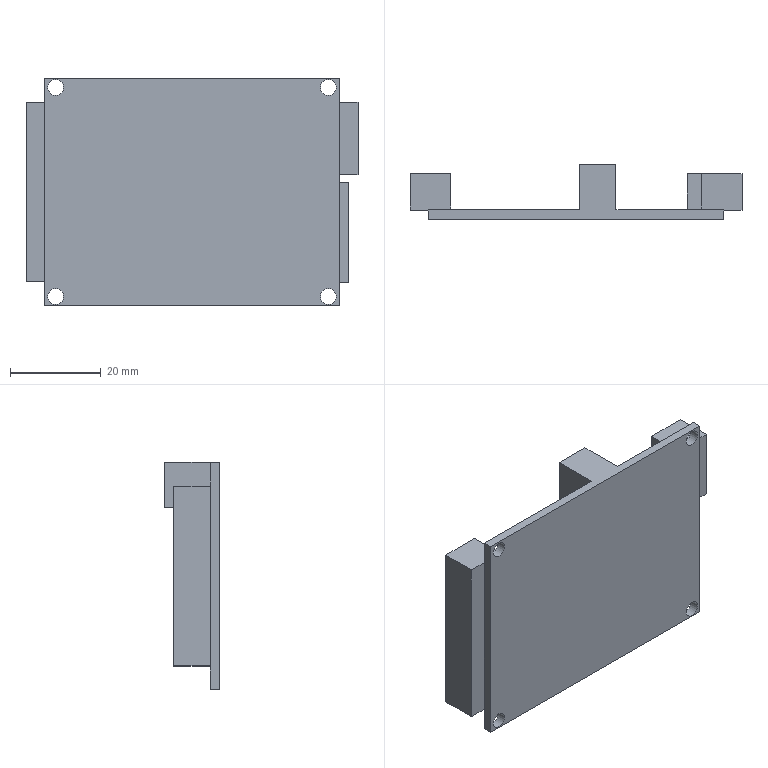Part | NX | features BREP 1 | 1 solid | 32 faces | box 73 x 12 x 50 mm | volume 12980 mm3 | plane 28 | cylinder 4 | commonest cylinder face diameters 3.5 x4
STEP:
#1=CARTESIAN_POINT('',(30.,2.,21.25));
#2=VERTEX_POINT('',#1);
#3=CARTESIAN_POINT('',(30.,2.,23.));
#4=DIRECTION('',(0.,1.,0.));
#5=DIRECTION('',(0.,0.,-1.));
#6=AXIS2_PLACEMENT_3D('',#3,#4,#5);
#7=CIRCLE('',#6,1.75);
#8=EDGE_CURVE('',#2,#2,#7,.T.);
#9=ORIENTED_EDGE('',*,*,#8,.T.);
#10=EDGE_LOOP('',(#9));
#11=FACE_BOUND('',#10,.T.);
#12=CARTESIAN_POINT('',(30.,0.,21.25));
#13=VERTEX_POINT('',#12);
#14=CARTESIAN_POINT('',(30.,0.,23.));
#15=DIRECTION('',(0.,1.,0.));
#16=DIRECTION('',(0.,0.,-1.));
#17=AXIS2_PLACEMENT_3D('',#14,#15,#16);
#18=CIRCLE('',#17,1.75);
#19=EDGE_CURVE('',#13,#13,#18,.T.);
#20=ORIENTED_EDGE('',*,*,#19,.F.);
#21=EDGE_LOOP('',(#20));
#22=FACE_BOUND('',#21,.T.);
#23=CARTESIAN_POINT('',(30.,0.,23.));
#24=DIRECTION('',(0.,1.,0.));
#25=DIRECTION('',(0.,0.,1.));
#26=AXIS2_PLACEMENT_3D('',#23,#24,#25);
#27=CYLINDRICAL_SURFACE('',#26,1.75);
#28=ADVANCED_FACE('',(#11,#22),#27,.F.);
#29=CARTESIAN_POINT('',(-30.,2.,24.75));
#30=VERTEX_POINT('',#29);
#31=CARTESIAN_POINT('',(-30.,2.,23.));
#32=DIRECTION('',(0.,1.,0.));
#33=DIRECTION('',(0.,0.,1.));
#34=AXIS2_PLACEMENT_3D('',#31,#32,#33);
#35=CIRCLE('',#34,1.75);
#36=EDGE_CURVE('',#30,#30,#35,.T.);
#37=ORIENTED_EDGE('',*,*,#36,.T.);
#38=EDGE_LOOP('',(#37));
#39=FACE_BOUND('',#38,.T.);
#40=CARTESIAN_POINT('',(-30.,0.,24.75));
#41=VERTEX_POINT('',#40);
#42=CARTESIAN_POINT('',(-30.,0.,23.));
#43=DIRECTION('',(0.,1.,0.));
#44=DIRECTION('',(0.,0.,1.));
#45=AXIS2_PLACEMENT_3D('',#42,#43,#44);
#46=CIRCLE('',#45,1.75);
#47=EDGE_CURVE('',#41,#41,#46,.T.);
#48=ORIENTED_EDGE('',*,*,#47,.F.);
#49=EDGE_LOOP('',(#48));
#50=FACE_BOUND('',#49,.T.);
#51=CARTESIAN_POINT('',(-30.,0.,23.));
#52=DIRECTION('',(0.,1.,0.));
#53=DIRECTION('',(0.,0.,1.));
#54=AXIS2_PLACEMENT_3D('',#51,#52,#53);
#55=CYLINDRICAL_SURFACE('',#54,1.75);
#56=ADVANCED_FACE('',(#39,#50),#55,.F.);
#57=CARTESIAN_POINT('',(-30.,2.,-24.75));
#58=VERTEX_POINT('',#57);
#59=CARTESIAN_POINT('',(-30.,2.,-23.));
#60=DIRECTION('',(0.,1.,0.));
#61=DIRECTION('',(0.,0.,-1.));
#62=AXIS2_PLACEMENT_3D('',#59,#60,#61);
#63=CIRCLE('',#62,1.75);
#64=EDGE_CURVE('',#58,#58,#63,.T.);
#65=ORIENTED_EDGE('',*,*,#64,.T.);
#66=EDGE_LOOP('',(#65));
#67=FACE_BOUND('',#66,.T.);
#68=CARTESIAN_POINT('',(-30.,0.,-24.75));
#69=VERTEX_POINT('',#68);
#70=CARTESIAN_POINT('',(-30.,0.,-23.));
#71=DIRECTION('',(0.,1.,0.));
#72=DIRECTION('',(0.,0.,-1.));
#73=AXIS2_PLACEMENT_3D('',#70,#71,#72);
#74=CIRCLE('',#73,1.75);
#75=EDGE_CURVE('',#69,#69,#74,.T.);
#76=ORIENTED_EDGE('',*,*,#75,.F.);
#77=EDGE_LOOP('',(#76));
#78=FACE_BOUND('',#77,.T.);
#79=CARTESIAN_POINT('',(-30.,0.,-23.));
#80=DIRECTION('',(0.,1.,0.));
#81=DIRECTION('',(0.,0.,1.));
#82=AXIS2_PLACEMENT_3D('',#79,#80,#81);
#83=CYLINDRICAL_SURFACE('',#82,1.75);
#84=ADVANCED_FACE('',(#67,#78),#83,.F.);
#85=CARTESIAN_POINT('',(30.,2.,-21.25));
#86=VERTEX_POINT('',#85);
#87=CARTESIAN_POINT('',(30.,2.,-23.));
#88=DIRECTION('',(0.,1.,0.));
#89=DIRECTION('',(0.,0.,1.));
#90=AXIS2_PLACEMENT_3D('',#87,#88,#89);
#91=CIRCLE('',#90,1.75);
#92=EDGE_CURVE('',#86,#86,#91,.T.);
#93=ORIENTED_EDGE('',*,*,#92,.T.);
#94=EDGE_LOOP('',(#93));
#95=FACE_BOUND('',#94,.T.);
#96=CARTESIAN_POINT('',(30.,0.,-21.25));
#97=VERTEX_POINT('',#96);
#98=CARTESIAN_POINT('',(30.,0.,-23.));
#99=DIRECTION('',(0.,1.,0.));
#100=DIRECTION('',(0.,0.,1.));
#101=AXIS2_PLACEMENT_3D('',#98,#99,#100);
#102=CIRCLE('',#101,1.75);
#103=EDGE_CURVE('',#97,#97,#102,.T.);
#104=ORIENTED_EDGE('',*,*,#103,.F.);
#105=EDGE_LOOP('',(#104));
#106=FACE_BOUND('',#105,.T.);
#107=CARTESIAN_POINT('',(30.,0.,-23.));
#108=DIRECTION('',(0.,1.,0.));
#109=DIRECTION('',(0.,0.,1.));
#110=AXIS2_PLACEMENT_3D('',#107,#108,#109);
#111=CYLINDRICAL_SURFACE('',#110,1.75);
#112=ADVANCED_FACE('',(#95,#106),#111,.F.);
#113=ORIENTED_EDGE('',*,*,#92,.F.);
#114=EDGE_LOOP('',(#113));
#115=FACE_BOUND('',#114,.T.);
#116=ORIENTED_EDGE('',*,*,#64,.F.);
#117=EDGE_LOOP('',(#116));
#118=FACE_BOUND('',#117,.T.);
#119=ORIENTED_EDGE('',*,*,#36,.F.);
#120=EDGE_LOOP('',(#119));
#121=FACE_BOUND('',#120,.T.);
#122=ORIENTED_EDGE('',*,*,#8,.F.);
#123=EDGE_LOOP('',(#122));
#124=FACE_BOUND('',#123,.T.);
#125=CARTESIAN_POINT('',(-32.5,2.,25.));
#126=VERTEX_POINT('',#125);
#127=CARTESIAN_POINT('',(0.7928,2.,25.));
#128=VERTEX_POINT('',#127);
#129=CARTESIAN_POINT('',(-32.5,2.,25.));
#130=DIRECTION('',(1.,0.,0.));
#131=VECTOR('',#130,1000.);
#132=LINE('',#129,#131);
#133=EDGE_CURVE('',#126,#128,#132,.T.);
#134=ORIENTED_EDGE('',*,*,#133,.T.);
#135=CARTESIAN_POINT('',(0.7928,2.,15.));
#136=VERTEX_POINT('',#135);
#137=CARTESIAN_POINT('',(0.7928,2.,15.));
#138=DIRECTION('',(0.,0.,1.));
#139=VECTOR('',#138,1000.);
#140=LINE('',#137,#139);
#141=EDGE_CURVE('',#136,#128,#140,.T.);
#142=ORIENTED_EDGE('',*,*,#141,.F.);
#143=CARTESIAN_POINT('',(8.793,2.,15.));
#144=VERTEX_POINT('',#143);
#145=CARTESIAN_POINT('',(0.7928,2.,15.));
#146=DIRECTION('',(-1.,0.,0.));
#147=VECTOR('',#146,1000.);
#148=LINE('',#145,#147);
#149=EDGE_CURVE('',#144,#136,#148,.T.);
#150=ORIENTED_EDGE('',*,*,#149,.F.);
#151=CARTESIAN_POINT('',(8.793,2.,25.));
#152=VERTEX_POINT('',#151);
#153=CARTESIAN_POINT('',(8.793,2.,15.));
#154=DIRECTION('',(0.,0.,-1.));
#155=VECTOR('',#154,1000.);
#156=LINE('',#153,#155);
#157=EDGE_CURVE('',#152,#144,#156,.T.);
#158=ORIENTED_EDGE('',*,*,#157,.F.);
#159=CARTESIAN_POINT('',(32.5,2.,25.));
#160=VERTEX_POINT('',#159);
#161=CARTESIAN_POINT('',(-32.5,2.,25.));
#162=DIRECTION('',(1.,0.,0.));
#163=VECTOR('',#162,1000.);
#164=LINE('',#161,#163);
#165=EDGE_CURVE('',#152,#160,#164,.T.);
#166=ORIENTED_EDGE('',*,*,#165,.T.);
#167=CARTESIAN_POINT('',(32.5,2.,19.756));
#168=VERTEX_POINT('',#167);
#169=CARTESIAN_POINT('',(32.5,2.,-25.));
#170=DIRECTION('',(0.,0.,-1.));
#171=VECTOR('',#170,1000.);
#172=LINE('',#169,#171);
#173=EDGE_CURVE('',#160,#168,#172,.T.);
#174=ORIENTED_EDGE('',*,*,#173,.T.);
#175=CARTESIAN_POINT('',(27.5,2.,19.756));
#176=VERTEX_POINT('',#175);
#177=CARTESIAN_POINT('',(27.5,2.,19.756));
#178=DIRECTION('',(1.,0.,0.));
#179=VECTOR('',#178,1000.);
#180=LINE('',#177,#179);
#181=EDGE_CURVE('',#176,#168,#180,.T.);
#182=ORIENTED_EDGE('',*,*,#181,.F.);
#183=CARTESIAN_POINT('',(27.5,2.,3.756));
#184=VERTEX_POINT('',#183);
#185=CARTESIAN_POINT('',(27.5,2.,19.756));
#186=DIRECTION('',(0.,0.,1.));
#187=VECTOR('',#186,1000.);
#188=LINE('',#185,#187);
#189=EDGE_CURVE('',#184,#176,#188,.T.);
#190=ORIENTED_EDGE('',*,*,#189,.F.);
#191=CARTESIAN_POINT('',(32.5,2.,3.756));
#192=VERTEX_POINT('',#191);
#193=CARTESIAN_POINT('',(0.,2.,3.756));
#194=DIRECTION('',(1.,0.,0.));
#195=VECTOR('',#194,1000.);
#196=LINE('',#193,#195);
#197=EDGE_CURVE('',#184,#192,#196,.T.);
#198=ORIENTED_EDGE('',*,*,#197,.T.);
#199=CARTESIAN_POINT('',(32.5,2.,2.163));
#200=VERTEX_POINT('',#199);
#201=CARTESIAN_POINT('',(32.5,2.,-25.));
#202=DIRECTION('',(0.,0.,-1.));
#203=VECTOR('',#202,1000.);
#204=LINE('',#201,#203);
#205=EDGE_CURVE('',#192,#200,#204,.T.);
#206=ORIENTED_EDGE('',*,*,#205,.T.);
#207=CARTESIAN_POINT('',(24.5,2.,2.163));
#208=VERTEX_POINT('',#207);
#209=CARTESIAN_POINT('',(24.5,2.,2.163));
#210=DIRECTION('',(1.,0.,0.));
#211=VECTOR('',#210,1000.);
#212=LINE('',#209,#211);
#213=EDGE_CURVE('',#208,#200,#212,.T.);
#214=ORIENTED_EDGE('',*,*,#213,.F.);
#215=CARTESIAN_POINT('',(24.5,2.,-19.837));
#216=VERTEX_POINT('',#215);
#217=CARTESIAN_POINT('',(24.5,2.,-19.837));
#218=DIRECTION('',(0.,0.,1.));
#219=VECTOR('',#218,1000.);
#220=LINE('',#217,#219);
#221=EDGE_CURVE('',#216,#208,#220,.T.);
#222=ORIENTED_EDGE('',*,*,#221,.F.);
#223=CARTESIAN_POINT('',(32.5,2.,-19.837));
#224=VERTEX_POINT('',#223);
#225=CARTESIAN_POINT('',(24.5,2.,-19.837));
#226=DIRECTION('',(-1.,0.,0.));
#227=VECTOR('',#226,1000.);
#228=LINE('',#225,#227);
#229=EDGE_CURVE('',#224,#216,#228,.T.);
#230=ORIENTED_EDGE('',*,*,#229,.F.);
#231=CARTESIAN_POINT('',(32.5,2.,-25.));
#232=VERTEX_POINT('',#231);
#233=CARTESIAN_POINT('',(32.5,2.,-25.));
#234=DIRECTION('',(0.,0.,-1.));
#235=VECTOR('',#234,1000.);
#236=LINE('',#233,#235);
#237=EDGE_CURVE('',#224,#232,#236,.T.);
#238=ORIENTED_EDGE('',*,*,#237,.T.);
#239=CARTESIAN_POINT('',(-32.5,2.,-25.));
#240=VERTEX_POINT('',#239);
#241=CARTESIAN_POINT('',(-32.5,2.,-25.));
#242=DIRECTION('',(-1.,0.,0.));
#243=VECTOR('',#242,1000.);
#244=LINE('',#241,#243);
#245=EDGE_CURVE('',#232,#240,#244,.T.);
#246=ORIENTED_EDGE('',*,*,#245,.T.);
#247=CARTESIAN_POINT('',(-32.5,2.,-19.756));
#248=VERTEX_POINT('',#247);
#249=CARTESIAN_POINT('',(-32.5,2.,-25.));
#250=DIRECTION('',(0.,0.,1.));
#251=VECTOR('',#250,1000.);
#252=LINE('',#249,#251);
#253=EDGE_CURVE('',#240,#248,#252,.T.);
#254=ORIENTED_EDGE('',*,*,#253,.T.);
#255=CARTESIAN_POINT('',(-27.5,2.,-19.756));
#256=VERTEX_POINT('',#255);
#257=CARTESIAN_POINT('',(-36.5,2.,-19.756));
#258=DIRECTION('',(-1.,0.,0.));
#259=VECTOR('',#258,1000.);
#260=LINE('',#257,#259);
#261=EDGE_CURVE('',#256,#248,#260,.T.);
#262=ORIENTED_EDGE('',*,*,#261,.F.);
#263=CARTESIAN_POINT('',(-27.5,2.,19.756));
#264=VERTEX_POINT('',#263);
#265=CARTESIAN_POINT('',(-27.5,2.,-19.756));
#266=DIRECTION('',(0.,0.,-1.));
#267=VECTOR('',#266,1000.);
#268=LINE('',#265,#267);
#269=EDGE_CURVE('',#264,#256,#268,.T.);
#270=ORIENTED_EDGE('',*,*,#269,.F.);
#271=CARTESIAN_POINT('',(-32.5,2.,19.756));
#272=VERTEX_POINT('',#271);
#273=CARTESIAN_POINT('',(-36.5,2.,19.756));
#274=DIRECTION('',(1.,0.,0.));
#275=VECTOR('',#274,1000.);
#276=LINE('',#273,#275);
#277=EDGE_CURVE('',#272,#264,#276,.T.);
#278=ORIENTED_EDGE('',*,*,#277,.F.);
#279=CARTESIAN_POINT('',(-32.5,2.,-25.));
#280=DIRECTION('',(0.,0.,1.));
#281=VECTOR('',#280,1000.);
#282=LINE('',#279,#281);
#283=EDGE_CURVE('',#272,#126,#282,.T.);
#284=ORIENTED_EDGE('',*,*,#283,.T.);
#285=EDGE_LOOP('',(#134,#142,#150,#158,#166,#174,#182,#190,#198,#206,#214,#222,#230,#238,#246,#254,#262,#270,#278,#284));
#286=FACE_BOUND('',#285,.T.);
#287=CARTESIAN_POINT('',(0.,2.,0.));
#288=DIRECTION('',(0.,1.,0.));
#289=DIRECTION('',(0.,0.,1.));
#290=AXIS2_PLACEMENT_3D('',#287,#288,#289);
#291=PLANE('',#290);
#292=ADVANCED_FACE('',(#115,#118,#121,#124,#286),#291,.T.);
#293=CARTESIAN_POINT('',(32.5,0.,25.));
#294=VERTEX_POINT('',#293);
#295=CARTESIAN_POINT('',(32.5,0.,-25.));
#296=VERTEX_POINT('',#295);
#297=CARTESIAN_POINT('',(32.5,0.,-25.));
#298=DIRECTION('',(0.,0.,-1.));
#299=VECTOR('',#298,1000.);
#300=LINE('',#297,#299);
#301=EDGE_CURVE('',#294,#296,#300,.T.);
#302=ORIENTED_EDGE('',*,*,#301,.T.);
#303=CARTESIAN_POINT('',(32.5,2.,-25.));
#304=DIRECTION('',(0.,-1.,0.));
#305=VECTOR('',#304,1000.);
#306=LINE('',#303,#305);
#307=EDGE_CURVE('',#232,#296,#306,.T.);
#308=ORIENTED_EDGE('',*,*,#307,.F.);
#309=ORIENTED_EDGE('',*,*,#237,.F.);
#310=CARTESIAN_POINT('',(32.5,2.,-25.));
#311=DIRECTION('',(0.,0.,-1.));
#312=VECTOR('',#311,1000.);
#313=LINE('',#310,#312);
#314=EDGE_CURVE('',#200,#224,#313,.T.);
#315=ORIENTED_EDGE('',*,*,#314,.F.);
#316=ORIENTED_EDGE('',*,*,#205,.F.);
#317=CARTESIAN_POINT('',(32.5,2.,-25.));
#318=DIRECTION('',(0.,0.,-1.));
#319=VECTOR('',#318,1000.);
#320=LINE('',#317,#319);
#321=EDGE_CURVE('',#168,#192,#320,.T.);
#322=ORIENTED_EDGE('',*,*,#321,.F.);
#323=ORIENTED_EDGE('',*,*,#173,.F.);
#324=CARTESIAN_POINT('',(32.5,2.,25.));
#325=DIRECTION('',(0.,-1.,0.));
#326=VECTOR('',#325,1000.);
#327=LINE('',#324,#326);
#328=EDGE_CURVE('',#160,#294,#327,.T.);
#329=ORIENTED_EDGE('',*,*,#328,.T.);
#330=EDGE_LOOP('',(#302,#308,#309,#315,#316,#322,#323,#329));
#331=FACE_BOUND('',#330,.T.);
#332=CARTESIAN_POINT('',(32.5,2.,-25.));
#333=DIRECTION('',(-1.,0.,0.));
#334=DIRECTION('',(0.,0.,1.));
#335=AXIS2_PLACEMENT_3D('',#332,#333,#334);
#336=PLANE('',#335);
#337=ADVANCED_FACE('',(#331),#336,.F.);
#338=CARTESIAN_POINT('',(-32.5,0.,-25.));
#339=VERTEX_POINT('',#338);
#340=CARTESIAN_POINT('',(-32.5,0.,-25.));
#341=DIRECTION('',(-1.,0.,0.));
#342=VECTOR('',#341,1000.);
#343=LINE('',#340,#342);
#344=EDGE_CURVE('',#296,#339,#343,.T.);
#345=ORIENTED_EDGE('',*,*,#344,.T.);
#346=CARTESIAN_POINT('',(-32.5,2.,-25.));
#347=DIRECTION('',(0.,-1.,0.));
#348=VECTOR('',#347,1000.);
#349=LINE('',#346,#348);
#350=EDGE_CURVE('',#240,#339,#349,.T.);
#351=ORIENTED_EDGE('',*,*,#350,.F.);
#352=ORIENTED_EDGE('',*,*,#245,.F.);
#353=ORIENTED_EDGE('',*,*,#307,.T.);
#354=EDGE_LOOP('',(#345,#351,#352,#353));
#355=FACE_BOUND('',#354,.T.);
#356=CARTESIAN_POINT('',(-32.5,2.,-25.));
#357=DIRECTION('',(0.,0.,1.));
#358=DIRECTION('',(1.,0.,0.));
#359=AXIS2_PLACEMENT_3D('',#356,#357,#358);
#360=PLANE('',#359);
#361=ADVANCED_FACE('',(#355),#360,.F.);
#362=CARTESIAN_POINT('',(-32.5,0.,25.));
#363=VERTEX_POINT('',#362);
#364=CARTESIAN_POINT('',(-32.5,0.,-25.));
#365=DIRECTION('',(0.,0.,1.));
#366=VECTOR('',#365,1000.);
#367=LINE('',#364,#366);
#368=EDGE_CURVE('',#339,#363,#367,.T.);
#369=ORIENTED_EDGE('',*,*,#368,.T.);
#370=CARTESIAN_POINT('',(-32.5,2.,25.));
#371=DIRECTION('',(0.,-1.,0.));
#372=VECTOR('',#371,1000.);
#373=LINE('',#370,#372);
#374=EDGE_CURVE('',#126,#363,#373,.T.);
#375=ORIENTED_EDGE('',*,*,#374,.F.);
#376=ORIENTED_EDGE('',*,*,#283,.F.);
#377=CARTESIAN_POINT('',(-32.5,2.,-25.));
#378=DIRECTION('',(0.,0.,1.));
#379=VECTOR('',#378,1000.);
#380=LINE('',#377,#379);
#381=EDGE_CURVE('',#248,#272,#380,.T.);
#382=ORIENTED_EDGE('',*,*,#381,.F.);
#383=ORIENTED_EDGE('',*,*,#253,.F.);
#384=ORIENTED_EDGE('',*,*,#350,.T.);
#385=EDGE_LOOP('',(#369,#375,#376,#382,#383,#384));
#386=FACE_BOUND('',#385,.T.);
#387=CARTESIAN_POINT('',(-32.5,2.,-25.));
#388=DIRECTION('',(1.,0.,0.));
#389=DIRECTION('',(0.,0.,-1.));
#390=AXIS2_PLACEMENT_3D('',#387,#388,#389);
#391=PLANE('',#390);
#392=ADVANCED_FACE('',(#386),#391,.F.);
#393=CARTESIAN_POINT('',(-32.5,0.,25.));
#394=DIRECTION('',(1.,0.,0.));
#395=VECTOR('',#394,1000.);
#396=LINE('',#393,#395);
#397=EDGE_CURVE('',#363,#294,#396,.T.);
#398=ORIENTED_EDGE('',*,*,#397,.T.);
#399=ORIENTED_EDGE('',*,*,#328,.F.);
#400=ORIENTED_EDGE('',*,*,#165,.F.);
#401=CARTESIAN_POINT('',(8.793,12.,25.));
#402=VERTEX_POINT('',#401);
#403=CARTESIAN_POINT('',(8.793,12.,25.));
#404=DIRECTION('',(0.,-1.,0.));
#405=VECTOR('',#404,1000.);
#406=LINE('',#403,#405);
#407=EDGE_CURVE('',#402,#152,#406,.T.);
#408=ORIENTED_EDGE('',*,*,#407,.F.);
#409=CARTESIAN_POINT('',(0.7928,12.,25.));
#410=VERTEX_POINT('',#409);
#411=CARTESIAN_POINT('',(0.7928,12.,25.));
#412=DIRECTION('',(1.,0.,0.));
#413=VECTOR('',#412,1000.);
#414=LINE('',#411,#413);
#415=EDGE_CURVE('',#410,#402,#414,.T.);
#416=ORIENTED_EDGE('',*,*,#415,.F.);
#417=CARTESIAN_POINT('',(0.7928,12.,25.));
#418=DIRECTION('',(0.,-1.,0.));
#419=VECTOR('',#418,1000.);
#420=LINE('',#417,#419);
#421=EDGE_CURVE('',#410,#128,#420,.T.);
#422=ORIENTED_EDGE('',*,*,#421,.T.);
#423=ORIENTED_EDGE('',*,*,#133,.F.);
#424=ORIENTED_EDGE('',*,*,#374,.T.);
#425=EDGE_LOOP('',(#398,#399,#400,#408,#416,#422,#423,#424));
#426=FACE_BOUND('',#425,.T.);
#427=CARTESIAN_POINT('',(-32.5,2.,25.));
#428=DIRECTION('',(0.,0.,-1.));
#429=DIRECTION('',(-1.,0.,0.));
#430=AXIS2_PLACEMENT_3D('',#427,#428,#429);
#431=PLANE('',#430);
#432=ADVANCED_FACE('',(#426),#431,.F.);
#433=ORIENTED_EDGE('',*,*,#19,.T.);
#434=EDGE_LOOP('',(#433));
#435=FACE_BOUND('',#434,.T.);
#436=ORIENTED_EDGE('',*,*,#47,.T.);
#437=EDGE_LOOP('',(#436));
#438=FACE_BOUND('',#437,.T.);
#439=ORIENTED_EDGE('',*,*,#75,.T.);
#440=EDGE_LOOP('',(#439));
#441=FACE_BOUND('',#440,.T.);
#442=ORIENTED_EDGE('',*,*,#103,.T.);
#443=EDGE_LOOP('',(#442));
#444=FACE_BOUND('',#443,.T.);
#445=ORIENTED_EDGE('',*,*,#301,.F.);
#446=ORIENTED_EDGE('',*,*,#397,.F.);
#447=ORIENTED_EDGE('',*,*,#368,.F.);
#448=ORIENTED_EDGE('',*,*,#344,.F.);
#449=EDGE_LOOP('',(#445,#446,#447,#448));
#450=FACE_BOUND('',#449,.T.);
#451=CARTESIAN_POINT('',(0.,0.,0.));
#452=DIRECTION('',(0.,1.,0.));
#453=DIRECTION('',(0.,0.,1.));
#454=AXIS2_PLACEMENT_3D('',#451,#452,#453);
#455=PLANE('',#454);
#456=ADVANCED_FACE('',(#435,#438,#441,#444,#450),#455,.F.);
#457=CARTESIAN_POINT('',(-36.5,2.,-19.756));
#458=VERTEX_POINT('',#457);
#459=CARTESIAN_POINT('',(-36.5,2.,-19.756));
#460=DIRECTION('',(-1.,0.,0.));
#461=VECTOR('',#460,1000.);
#462=LINE('',#459,#461);
#463=EDGE_CURVE('',#248,#458,#462,.T.);
#464=ORIENTED_EDGE('',*,*,#463,.F.);
#465=ORIENTED_EDGE('',*,*,#381,.T.);
#466=CARTESIAN_POINT('',(-36.5,2.,19.756));
#467=VERTEX_POINT('',#466);
#468=CARTESIAN_POINT('',(-36.5,2.,19.756));
#469=DIRECTION('',(1.,0.,0.));
#470=VECTOR('',#469,1000.);
#471=LINE('',#468,#470);
#472=EDGE_CURVE('',#467,#272,#471,.T.);
#473=ORIENTED_EDGE('',*,*,#472,.F.);
#474=CARTESIAN_POINT('',(-36.5,2.,-19.756));
#475=DIRECTION('',(0.,0.,1.));
#476=VECTOR('',#475,1000.);
#477=LINE('',#474,#476);
#478=EDGE_CURVE('',#458,#467,#477,.T.);
#479=ORIENTED_EDGE('',*,*,#478,.F.);
#480=EDGE_LOOP('',(#464,#465,#473,#479));
#481=FACE_BOUND('',#480,.T.);
#482=CARTESIAN_POINT('',(0.,2.,0.));
#483=DIRECTION('',(0.,1.,0.));
#484=DIRECTION('',(0.,0.,1.));
#485=AXIS2_PLACEMENT_3D('',#482,#483,#484);
#486=PLANE('',#485);
#487=ADVANCED_FACE('',(#481),#486,.F.);
#488=ORIENTED_EDGE('',*,*,#478,.T.);
#489=CARTESIAN_POINT('',(-36.5,10.,19.756));
#490=VERTEX_POINT('',#489);
#491=CARTESIAN_POINT('',(-36.5,10.,19.756));
#492=DIRECTION('',(0.,-1.,0.));
#493=VECTOR('',#492,1000.);
#494=LINE('',#491,#493);
#495=EDGE_CURVE('',#490,#467,#494,.T.);
#496=ORIENTED_EDGE('',*,*,#495,.F.);
#497=CARTESIAN_POINT('',(-36.5,10.,-19.756));
#498=VERTEX_POINT('',#497);
#499=CARTESIAN_POINT('',(-36.5,10.,-19.756));
#500=DIRECTION('',(0.,0.,1.));
#501=VECTOR('',#500,1000.);
#502=LINE('',#499,#501);
#503=EDGE_CURVE('',#498,#490,#502,.T.);
#504=ORIENTED_EDGE('',*,*,#503,.F.);
#505=CARTESIAN_POINT('',(-36.5,10.,-19.756));
#506=DIRECTION('',(0.,-1.,0.));
#507=VECTOR('',#506,1000.);
#508=LINE('',#505,#507);
#509=EDGE_CURVE('',#498,#458,#508,.T.);
#510=ORIENTED_EDGE('',*,*,#509,.T.);
#511=EDGE_LOOP('',(#488,#496,#504,#510));
#512=FACE_BOUND('',#511,.T.);
#513=CARTESIAN_POINT('',(-36.5,10.,-19.756));
#514=DIRECTION('',(1.,0.,0.));
#515=DIRECTION('',(0.,0.,-1.));
#516=AXIS2_PLACEMENT_3D('',#513,#514,#515);
#517=PLANE('',#516);
#518=ADVANCED_FACE('',(#512),#517,.F.);
#519=ORIENTED_EDGE('',*,*,#472,.T.);
#520=ORIENTED_EDGE('',*,*,#277,.T.);
#521=CARTESIAN_POINT('',(-27.5,10.,19.756));
#522=VERTEX_POINT('',#521);
#523=CARTESIAN_POINT('',(-27.5,10.,19.756));
#524=DIRECTION('',(0.,-1.,0.));
#525=VECTOR('',#524,1000.);
#526=LINE('',#523,#525);
#527=EDGE_CURVE('',#522,#264,#526,.T.);
#528=ORIENTED_EDGE('',*,*,#527,.F.);
#529=CARTESIAN_POINT('',(-36.5,10.,19.756));
#530=DIRECTION('',(1.,0.,0.));
#531=VECTOR('',#530,1000.);
#532=LINE('',#529,#531);
#533=EDGE_CURVE('',#490,#522,#532,.T.);
#534=ORIENTED_EDGE('',*,*,#533,.F.);
#535=ORIENTED_EDGE('',*,*,#495,.T.);
#536=EDGE_LOOP('',(#519,#520,#528,#534,#535));
#537=FACE_BOUND('',#536,.T.);
#538=CARTESIAN_POINT('',(-36.5,10.,19.756));
#539=DIRECTION('',(0.,0.,-1.));
#540=DIRECTION('',(-1.,0.,0.));
#541=AXIS2_PLACEMENT_3D('',#538,#539,#540);
#542=PLANE('',#541);
#543=ADVANCED_FACE('',(#537),#542,.F.);
#544=ORIENTED_EDGE('',*,*,#269,.T.);
#545=CARTESIAN_POINT('',(-27.5,10.,-19.756));
#546=VERTEX_POINT('',#545);
#547=CARTESIAN_POINT('',(-27.5,10.,-19.756));
#548=DIRECTION('',(0.,-1.,0.));
#549=VECTOR('',#548,1000.);
#550=LINE('',#547,#549);
#551=EDGE_CURVE('',#546,#256,#550,.T.);
#552=ORIENTED_EDGE('',*,*,#551,.F.);
#553=CARTESIAN_POINT('',(-27.5,10.,-19.756));
#554=DIRECTION('',(0.,0.,-1.));
#555=VECTOR('',#554,1000.);
#556=LINE('',#553,#555);
#557=EDGE_CURVE('',#522,#546,#556,.T.);
#558=ORIENTED_EDGE('',*,*,#557,.F.);
#559=ORIENTED_EDGE('',*,*,#527,.T.);
#560=EDGE_LOOP('',(#544,#552,#558,#559));
#561=FACE_BOUND('',#560,.T.);
#562=CARTESIAN_POINT('',(-27.5,10.,-19.756));
#563=DIRECTION('',(-1.,0.,0.));
#564=DIRECTION('',(0.,0.,1.));
#565=AXIS2_PLACEMENT_3D('',#562,#563,#564);
#566=PLANE('',#565);
#567=ADVANCED_FACE('',(#561),#566,.F.);
#568=ORIENTED_EDGE('',*,*,#261,.T.);
#569=ORIENTED_EDGE('',*,*,#463,.T.);
#570=ORIENTED_EDGE('',*,*,#509,.F.);
#571=CARTESIAN_POINT('',(-36.5,10.,-19.756));
#572=DIRECTION('',(-1.,0.,0.));
#573=VECTOR('',#572,1000.);
#574=LINE('',#571,#573);
#575=EDGE_CURVE('',#546,#498,#574,.T.);
#576=ORIENTED_EDGE('',*,*,#575,.F.);
#577=ORIENTED_EDGE('',*,*,#551,.T.);
#578=EDGE_LOOP('',(#568,#569,#570,#576,#577));
#579=FACE_BOUND('',#578,.T.);
#580=CARTESIAN_POINT('',(-36.5,10.,-19.756));
#581=DIRECTION('',(0.,0.,1.));
#582=DIRECTION('',(1.,0.,0.));
#583=AXIS2_PLACEMENT_3D('',#580,#581,#582);
#584=PLANE('',#583);
#585=ADVANCED_FACE('',(#579),#584,.F.);
#586=ORIENTED_EDGE('',*,*,#503,.T.);
#587=ORIENTED_EDGE('',*,*,#533,.T.);
#588=ORIENTED_EDGE('',*,*,#557,.T.);
#589=ORIENTED_EDGE('',*,*,#575,.T.);
#590=EDGE_LOOP('',(#586,#587,#588,#589));
#591=FACE_BOUND('',#590,.T.);
#592=CARTESIAN_POINT('',(0.,10.,0.));
#593=DIRECTION('',(0.,1.,0.));
#594=DIRECTION('',(0.,0.,1.));
#595=AXIS2_PLACEMENT_3D('',#592,#593,#594);
#596=PLANE('',#595);
#597=ADVANCED_FACE('',(#591),#596,.T.);
#598=ORIENTED_EDGE('',*,*,#321,.T.);
#599=CARTESIAN_POINT('',(36.5,2.,3.756));
#600=VERTEX_POINT('',#599);
#601=CARTESIAN_POINT('',(27.5,2.,3.756));
#602=DIRECTION('',(-1.,0.,0.));
#603=VECTOR('',#602,1000.);
#604=LINE('',#601,#603);
#605=EDGE_CURVE('',#600,#192,#604,.T.);
#606=ORIENTED_EDGE('',*,*,#605,.F.);
#607=CARTESIAN_POINT('',(36.5,2.,19.756));
#608=VERTEX_POINT('',#607);
#609=CARTESIAN_POINT('',(36.5,2.,19.756));
#610=DIRECTION('',(0.,0.,-1.));
#611=VECTOR('',#610,1000.);
#612=LINE('',#609,#611);
#613=EDGE_CURVE('',#608,#600,#612,.T.);
#614=ORIENTED_EDGE('',*,*,#613,.F.);
#615=CARTESIAN_POINT('',(27.5,2.,19.756));
#616=DIRECTION('',(1.,0.,0.));
#617=VECTOR('',#616,1000.);
#618=LINE('',#615,#617);
#619=EDGE_CURVE('',#168,#608,#618,.T.);
#620=ORIENTED_EDGE('',*,*,#619,.F.);
#621=EDGE_LOOP('',(#598,#606,#614,#620));
#622=FACE_BOUND('',#621,.T.);
#623=CARTESIAN_POINT('',(0.,2.,0.));
#624=DIRECTION('',(0.,-1.,0.));
#625=DIRECTION('',(0.,0.,-1.));
#626=AXIS2_PLACEMENT_3D('',#623,#624,#625);
#627=PLANE('',#626);
#628=ADVANCED_FACE('',(#622),#627,.T.);
#629=ORIENTED_EDGE('',*,*,#189,.T.);
#630=CARTESIAN_POINT('',(27.5,10.,19.756));
#631=VERTEX_POINT('',#630);
#632=CARTESIAN_POINT('',(27.5,10.,19.756));
#633=DIRECTION('',(0.,-1.,0.));
#634=VECTOR('',#633,1000.);
#635=LINE('',#632,#634);
#636=EDGE_CURVE('',#631,#176,#635,.T.);
#637=ORIENTED_EDGE('',*,*,#636,.F.);
#638=CARTESIAN_POINT('',(27.5,10.,3.756));
#639=VERTEX_POINT('',#638);
#640=CARTESIAN_POINT('',(27.5,10.,19.756));
#641=DIRECTION('',(0.,0.,1.));
#642=VECTOR('',#641,1000.);
#643=LINE('',#640,#642);
#644=EDGE_CURVE('',#639,#631,#643,.T.);
#645=ORIENTED_EDGE('',*,*,#644,.F.);
#646=CARTESIAN_POINT('',(27.5,10.,3.756));
#647=DIRECTION('',(0.,-1.,0.));
#648=VECTOR('',#647,1000.);
#649=LINE('',#646,#648);
#650=EDGE_CURVE('',#639,#184,#649,.T.);
#651=ORIENTED_EDGE('',*,*,#650,.T.);
#652=EDGE_LOOP('',(#629,#637,#645,#651));
#653=FACE_BOUND('',#652,.T.);
#654=CARTESIAN_POINT('',(27.5,10.,19.756));
#655=DIRECTION('',(1.,0.,0.));
#656=DIRECTION('',(0.,0.,-1.));
#657=AXIS2_PLACEMENT_3D('',#654,#655,#656);
#658=PLANE('',#657);
#659=ADVANCED_FACE('',(#653),#658,.F.);
#660=ORIENTED_EDGE('',*,*,#181,.T.);
#661=ORIENTED_EDGE('',*,*,#619,.T.);
#662=CARTESIAN_POINT('',(36.5,10.,19.756));
#663=VERTEX_POINT('',#662);
#664=CARTESIAN_POINT('',(36.5,10.,19.756));
#665=DIRECTION('',(0.,-1.,0.));
#666=VECTOR('',#665,1000.);
#667=LINE('',#664,#666);
#668=EDGE_CURVE('',#663,#608,#667,.T.);
#669=ORIENTED_EDGE('',*,*,#668,.F.);
#670=CARTESIAN_POINT('',(27.5,10.,19.756));
#671=DIRECTION('',(1.,0.,0.));
#672=VECTOR('',#671,1000.);
#673=LINE('',#670,#672);
#674=EDGE_CURVE('',#631,#663,#673,.T.);
#675=ORIENTED_EDGE('',*,*,#674,.F.);
#676=ORIENTED_EDGE('',*,*,#636,.T.);
#677=EDGE_LOOP('',(#660,#661,#669,#675,#676));
#678=FACE_BOUND('',#677,.T.);
#679=CARTESIAN_POINT('',(27.5,10.,19.756));
#680=DIRECTION('',(0.,0.,-1.));
#681=DIRECTION('',(-1.,0.,0.));
#682=AXIS2_PLACEMENT_3D('',#679,#680,#681);
#683=PLANE('',#682);
#684=ADVANCED_FACE('',(#678),#683,.F.);
#685=ORIENTED_EDGE('',*,*,#613,.T.);
#686=CARTESIAN_POINT('',(36.5,10.,3.756));
#687=VERTEX_POINT('',#686);
#688=CARTESIAN_POINT('',(36.5,10.,3.756));
#689=DIRECTION('',(0.,-1.,0.));
#690=VECTOR('',#689,1000.);
#691=LINE('',#688,#690);
#692=EDGE_CURVE('',#687,#600,#691,.T.);
#693=ORIENTED_EDGE('',*,*,#692,.F.);
#694=CARTESIAN_POINT('',(36.5,10.,19.756));
#695=DIRECTION('',(0.,0.,-1.));
#696=VECTOR('',#695,1000.);
#697=LINE('',#694,#696);
#698=EDGE_CURVE('',#663,#687,#697,.T.);
#699=ORIENTED_EDGE('',*,*,#698,.F.);
#700=ORIENTED_EDGE('',*,*,#668,.T.);
#701=EDGE_LOOP('',(#685,#693,#699,#700));
#702=FACE_BOUND('',#701,.T.);
#703=CARTESIAN_POINT('',(36.5,10.,19.756));
#704=DIRECTION('',(-1.,0.,0.));
#705=DIRECTION('',(0.,0.,1.));
#706=AXIS2_PLACEMENT_3D('',#703,#704,#705);
#707=PLANE('',#706);
#708=ADVANCED_FACE('',(#702),#707,.F.);
#709=ORIENTED_EDGE('',*,*,#605,.T.);
#710=ORIENTED_EDGE('',*,*,#197,.F.);
#711=ORIENTED_EDGE('',*,*,#650,.F.);
#712=CARTESIAN_POINT('',(27.5,10.,3.756));
#713=DIRECTION('',(-1.,0.,0.));
#714=VECTOR('',#713,1000.);
#715=LINE('',#712,#714);
#716=EDGE_CURVE('',#687,#639,#715,.T.);
#717=ORIENTED_EDGE('',*,*,#716,.F.);
#718=ORIENTED_EDGE('',*,*,#692,.T.);
#719=EDGE_LOOP('',(#709,#710,#711,#717,#718));
#720=FACE_BOUND('',#719,.T.);
#721=CARTESIAN_POINT('',(27.5,10.,3.756));
#722=DIRECTION('',(0.,0.,1.));
#723=DIRECTION('',(1.,0.,0.));
#724=AXIS2_PLACEMENT_3D('',#721,#722,#723);
#725=PLANE('',#724);
#726=ADVANCED_FACE('',(#720),#725,.F.);
#727=ORIENTED_EDGE('',*,*,#644,.T.);
#728=ORIENTED_EDGE('',*,*,#674,.T.);
#729=ORIENTED_EDGE('',*,*,#698,.T.);
#730=ORIENTED_EDGE('',*,*,#716,.T.);
#731=EDGE_LOOP('',(#727,#728,#729,#730));
#732=FACE_BOUND('',#731,.T.);
#733=CARTESIAN_POINT('',(0.,10.,0.));
#734=DIRECTION('',(0.,-1.,0.));
#735=DIRECTION('',(0.,0.,-1.));
#736=AXIS2_PLACEMENT_3D('',#733,#734,#735);
#737=PLANE('',#736);
#738=ADVANCED_FACE('',(#732),#737,.F.);
#739=CARTESIAN_POINT('',(34.5,2.,2.163));
#740=VERTEX_POINT('',#739);
#741=CARTESIAN_POINT('',(24.5,2.,2.163));
#742=DIRECTION('',(1.,0.,0.));
#743=VECTOR('',#742,1000.);
#744=LINE('',#741,#743);
#745=EDGE_CURVE('',#200,#740,#744,.T.);
#746=ORIENTED_EDGE('',*,*,#745,.F.);
#747=ORIENTED_EDGE('',*,*,#314,.T.);
#748=CARTESIAN_POINT('',(34.5,2.,-19.837));
#749=VERTEX_POINT('',#748);
#750=CARTESIAN_POINT('',(24.5,2.,-19.837));
#751=DIRECTION('',(-1.,0.,0.));
#752=VECTOR('',#751,1000.);
#753=LINE('',#750,#752);
#754=EDGE_CURVE('',#749,#224,#753,.T.);
#755=ORIENTED_EDGE('',*,*,#754,.F.);
#756=CARTESIAN_POINT('',(34.5,2.,-19.837));
#757=DIRECTION('',(0.,0.,-1.));
#758=VECTOR('',#757,1000.);
#759=LINE('',#756,#758);
#760=EDGE_CURVE('',#740,#749,#759,.T.);
#761=ORIENTED_EDGE('',*,*,#760,.F.);
#762=EDGE_LOOP('',(#746,#747,#755,#761));
#763=FACE_BOUND('',#762,.T.);
#764=CARTESIAN_POINT('',(0.,2.,0.));
#765=DIRECTION('',(0.,1.,0.));
#766=DIRECTION('',(0.,0.,1.));
#767=AXIS2_PLACEMENT_3D('',#764,#765,#766);
#768=PLANE('',#767);
#769=ADVANCED_FACE('',(#763),#768,.F.);
#770=ORIENTED_EDGE('',*,*,#221,.T.);
#771=CARTESIAN_POINT('',(24.5,10.,2.163));
#772=VERTEX_POINT('',#771);
#773=CARTESIAN_POINT('',(24.5,10.,2.163));
#774=DIRECTION('',(0.,-1.,0.));
#775=VECTOR('',#774,1000.);
#776=LINE('',#773,#775);
#777=EDGE_CURVE('',#772,#208,#776,.T.);
#778=ORIENTED_EDGE('',*,*,#777,.F.);
#779=CARTESIAN_POINT('',(24.5,10.,-19.837));
#780=VERTEX_POINT('',#779);
#781=CARTESIAN_POINT('',(24.5,10.,-19.837));
#782=DIRECTION('',(0.,0.,1.));
#783=VECTOR('',#782,1000.);
#784=LINE('',#781,#783);
#785=EDGE_CURVE('',#780,#772,#784,.T.);
#786=ORIENTED_EDGE('',*,*,#785,.F.);
#787=CARTESIAN_POINT('',(24.5,10.,-19.837));
#788=DIRECTION('',(0.,-1.,0.));
#789=VECTOR('',#788,1000.);
#790=LINE('',#787,#789);
#791=EDGE_CURVE('',#780,#216,#790,.T.);
#792=ORIENTED_EDGE('',*,*,#791,.T.);
#793=EDGE_LOOP('',(#770,#778,#786,#792));
#794=FACE_BOUND('',#793,.T.);
#795=CARTESIAN_POINT('',(24.5,10.,-19.837));
#796=DIRECTION('',(1.,0.,0.));
#797=DIRECTION('',(0.,0.,-1.));
#798=AXIS2_PLACEMENT_3D('',#795,#796,#797);
#799=PLANE('',#798);
#800=ADVANCED_FACE('',(#794),#799,.F.);
#801=ORIENTED_EDGE('',*,*,#213,.T.);
#802=ORIENTED_EDGE('',*,*,#745,.T.);
#803=CARTESIAN_POINT('',(34.5,10.,2.163));
#804=VERTEX_POINT('',#803);
#805=CARTESIAN_POINT('',(34.5,10.,2.163));
#806=DIRECTION('',(0.,-1.,0.));
#807=VECTOR('',#806,1000.);
#808=LINE('',#805,#807);
#809=EDGE_CURVE('',#804,#740,#808,.T.);
#810=ORIENTED_EDGE('',*,*,#809,.F.);
#811=CARTESIAN_POINT('',(24.5,10.,2.163));
#812=DIRECTION('',(1.,0.,0.));
#813=VECTOR('',#812,1000.);
#814=LINE('',#811,#813);
#815=EDGE_CURVE('',#772,#804,#814,.T.);
#816=ORIENTED_EDGE('',*,*,#815,.F.);
#817=ORIENTED_EDGE('',*,*,#777,.T.);
#818=EDGE_LOOP('',(#801,#802,#810,#816,#817));
#819=FACE_BOUND('',#818,.T.);
#820=CARTESIAN_POINT('',(24.5,10.,2.163));
#821=DIRECTION('',(0.,0.,-1.));
#822=DIRECTION('',(-1.,0.,0.));
#823=AXIS2_PLACEMENT_3D('',#820,#821,#822);
#824=PLANE('',#823);
#825=ADVANCED_FACE('',(#819),#824,.F.);
#826=ORIENTED_EDGE('',*,*,#760,.T.);
#827=CARTESIAN_POINT('',(34.5,10.,-19.837));
#828=VERTEX_POINT('',#827);
#829=CARTESIAN_POINT('',(34.5,10.,-19.837));
#830=DIRECTION('',(0.,-1.,0.));
#831=VECTOR('',#830,1000.);
#832=LINE('',#829,#831);
#833=EDGE_CURVE('',#828,#749,#832,.T.);
#834=ORIENTED_EDGE('',*,*,#833,.F.);
#835=CARTESIAN_POINT('',(34.5,10.,-19.837));
#836=DIRECTION('',(0.,0.,-1.));
#837=VECTOR('',#836,1000.);
#838=LINE('',#835,#837);
#839=EDGE_CURVE('',#804,#828,#838,.T.);
#840=ORIENTED_EDGE('',*,*,#839,.F.);
#841=ORIENTED_EDGE('',*,*,#809,.T.);
#842=EDGE_LOOP('',(#826,#834,#840,#841));
#843=FACE_BOUND('',#842,.T.);
#844=CARTESIAN_POINT('',(34.5,10.,-19.837));
#845=DIRECTION('',(-1.,0.,0.));
#846=DIRECTION('',(0.,0.,1.));
#847=AXIS2_PLACEMENT_3D('',#844,#845,#846);
#848=PLANE('',#847);
#849=ADVANCED_FACE('',(#843),#848,.F.);
#850=ORIENTED_EDGE('',*,*,#754,.T.);
#851=ORIENTED_EDGE('',*,*,#229,.T.);
#852=ORIENTED_EDGE('',*,*,#791,.F.);
#853=CARTESIAN_POINT('',(24.5,10.,-19.837));
#854=DIRECTION('',(-1.,0.,0.));
#855=VECTOR('',#854,1000.);
#856=LINE('',#853,#855);
#857=EDGE_CURVE('',#828,#780,#856,.T.);
#858=ORIENTED_EDGE('',*,*,#857,.F.);
#859=ORIENTED_EDGE('',*,*,#833,.T.);
#860=EDGE_LOOP('',(#850,#851,#852,#858,#859));
#861=FACE_BOUND('',#860,.T.);
#862=CARTESIAN_POINT('',(24.5,10.,-19.837));
#863=DIRECTION('',(0.,0.,1.));
#864=DIRECTION('',(1.,0.,0.));
#865=AXIS2_PLACEMENT_3D('',#862,#863,#864);
#866=PLANE('',#865);
#867=ADVANCED_FACE('',(#861),#866,.F.);
#868=ORIENTED_EDGE('',*,*,#785,.T.);
#869=ORIENTED_EDGE('',*,*,#815,.T.);
#870=ORIENTED_EDGE('',*,*,#839,.T.);
#871=ORIENTED_EDGE('',*,*,#857,.T.);
#872=EDGE_LOOP('',(#868,#869,#870,#871));
#873=FACE_BOUND('',#872,.T.);
#874=CARTESIAN_POINT('',(0.,10.,0.));
#875=DIRECTION('',(0.,1.,0.));
#876=DIRECTION('',(0.,0.,1.));
#877=AXIS2_PLACEMENT_3D('',#874,#875,#876);
#878=PLANE('',#877);
#879=ADVANCED_FACE('',(#873),#878,.T.);
#880=ORIENTED_EDGE('',*,*,#141,.T.);
#881=ORIENTED_EDGE('',*,*,#421,.F.);
#882=CARTESIAN_POINT('',(0.7928,12.,15.));
#883=VERTEX_POINT('',#882);
#884=CARTESIAN_POINT('',(0.7928,12.,15.));
#885=DIRECTION('',(0.,0.,1.));
#886=VECTOR('',#885,1000.);
#887=LINE('',#884,#886);
#888=EDGE_CURVE('',#883,#410,#887,.T.);
#889=ORIENTED_EDGE('',*,*,#888,.F.);
#890=CARTESIAN_POINT('',(0.7928,12.,15.));
#891=DIRECTION('',(0.,-1.,0.));
#892=VECTOR('',#891,1000.);
#893=LINE('',#890,#892);
#894=EDGE_CURVE('',#883,#136,#893,.T.);
#895=ORIENTED_EDGE('',*,*,#894,.T.);
#896=EDGE_LOOP('',(#880,#881,#889,#895));
#897=FACE_BOUND('',#896,.T.);
#898=CARTESIAN_POINT('',(0.7928,12.,15.));
#899=DIRECTION('',(1.,0.,0.));
#900=DIRECTION('',(0.,0.,-1.));
#901=AXIS2_PLACEMENT_3D('',#898,#899,#900);
#902=PLANE('',#901);
#903=ADVANCED_FACE('',(#897),#902,.F.);
#904=ORIENTED_EDGE('',*,*,#157,.T.);
#905=CARTESIAN_POINT('',(8.793,12.,15.));
#906=VERTEX_POINT('',#905);
#907=CARTESIAN_POINT('',(8.793,12.,15.));
#908=DIRECTION('',(0.,-1.,0.));
#909=VECTOR('',#908,1000.);
#910=LINE('',#907,#909);
#911=EDGE_CURVE('',#906,#144,#910,.T.);
#912=ORIENTED_EDGE('',*,*,#911,.F.);
#913=CARTESIAN_POINT('',(8.793,12.,15.));
#914=DIRECTION('',(0.,0.,-1.));
#915=VECTOR('',#914,1000.);
#916=LINE('',#913,#915);
#917=EDGE_CURVE('',#402,#906,#916,.T.);
#918=ORIENTED_EDGE('',*,*,#917,.F.);
#919=ORIENTED_EDGE('',*,*,#407,.T.);
#920=EDGE_LOOP('',(#904,#912,#918,#919));
#921=FACE_BOUND('',#920,.T.);
#922=CARTESIAN_POINT('',(8.793,12.,15.));
#923=DIRECTION('',(-1.,0.,0.));
#924=DIRECTION('',(0.,0.,1.));
#925=AXIS2_PLACEMENT_3D('',#922,#923,#924);
#926=PLANE('',#925);
#927=ADVANCED_FACE('',(#921),#926,.F.);
#928=ORIENTED_EDGE('',*,*,#149,.T.);
#929=ORIENTED_EDGE('',*,*,#894,.F.);
#930=CARTESIAN_POINT('',(0.7928,12.,15.));
#931=DIRECTION('',(-1.,0.,0.));
#932=VECTOR('',#931,1000.);
#933=LINE('',#930,#932);
#934=EDGE_CURVE('',#906,#883,#933,.T.);
#935=ORIENTED_EDGE('',*,*,#934,.F.);
#936=ORIENTED_EDGE('',*,*,#911,.T.);
#937=EDGE_LOOP('',(#928,#929,#935,#936));
#938=FACE_BOUND('',#937,.T.);
#939=CARTESIAN_POINT('',(0.7928,12.,15.));
#940=DIRECTION('',(0.,0.,1.));
#941=DIRECTION('',(1.,0.,0.));
#942=AXIS2_PLACEMENT_3D('',#939,#940,#941);
#943=PLANE('',#942);
#944=ADVANCED_FACE('',(#938),#943,.F.);
#945=ORIENTED_EDGE('',*,*,#888,.T.);
#946=ORIENTED_EDGE('',*,*,#415,.T.);
#947=ORIENTED_EDGE('',*,*,#917,.T.);
#948=ORIENTED_EDGE('',*,*,#934,.T.);
#949=EDGE_LOOP('',(#945,#946,#947,#948));
#950=FACE_BOUND('',#949,.T.);
#951=CARTESIAN_POINT('',(0.,12.,0.));
#952=DIRECTION('',(0.,1.,0.));
#953=DIRECTION('',(0.,0.,1.));
#954=AXIS2_PLACEMENT_3D('',#951,#952,#953);
#955=PLANE('',#954);
#956=ADVANCED_FACE('',(#950),#955,.T.);
#957=CLOSED_SHELL('',(#28,#56,#84,#112,#292,#337,#361,#392,#432,#456,#487,#518,#543,#567,#585,#597,#628,#659,#684,#708,#726,#738,#769,#800,#825,#849,#867,#879,#903,#927,#944,#956));
#958=MANIFOLD_SOLID_BREP('',#957);
#959=(LENGTH_UNIT()NAMED_UNIT(*)SI_UNIT(.MILLI.,.METRE.));
#960=UNCERTAINTY_MEASURE_WITH_UNIT(LENGTH_MEASURE(0.00001),#959,'','');
#961=(NAMED_UNIT(*)PLANE_ANGLE_UNIT()SI_UNIT($,.RADIAN.));
#962=(NAMED_UNIT(*)SI_UNIT($,.STERADIAN.)SOLID_ANGLE_UNIT());
#963=(GEOMETRIC_REPRESENTATION_CONTEXT(3)GLOBAL_UNCERTAINTY_ASSIGNED_CONTEXT((#960))GLOBAL_UNIT_ASSIGNED_CONTEXT((#959,#961,#962))REPRESENTATION_CONTEXT('',''));
#964=ADVANCED_BREP_SHAPE_REPRESENTATION('',(#958),#963);